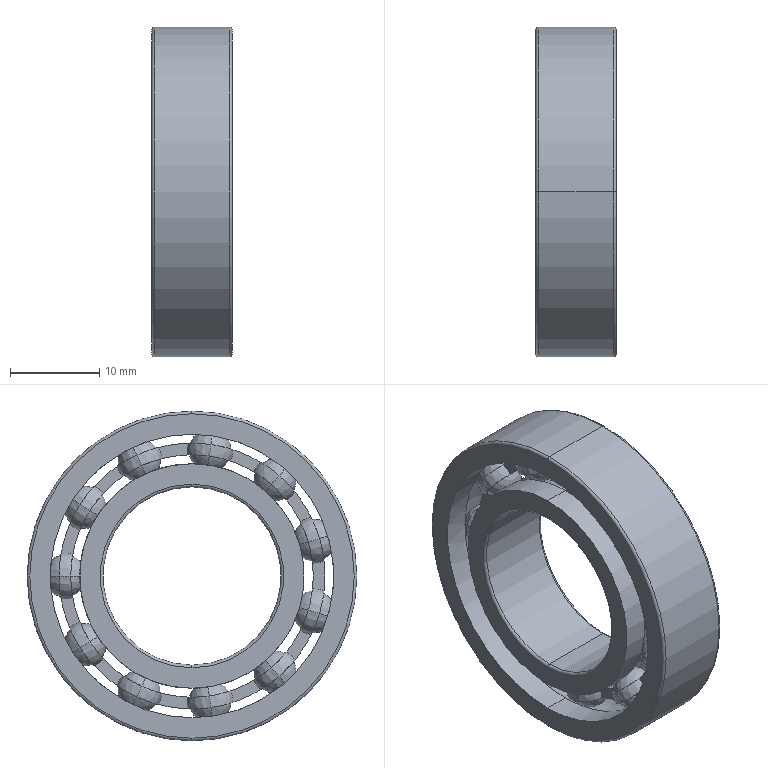Part | STEP file | Bearing 6904Z | 1 solid | 174 faces | box 9 x 37 x 37 mm | volume 4601 mm3 | sphere 88 | torus 44 | plane 26 | cylinder 16 | commonest cylinder face diameters 25.2 x4 31.8 x4 20 x2 27.19 x2 29.81 x2 37 x2